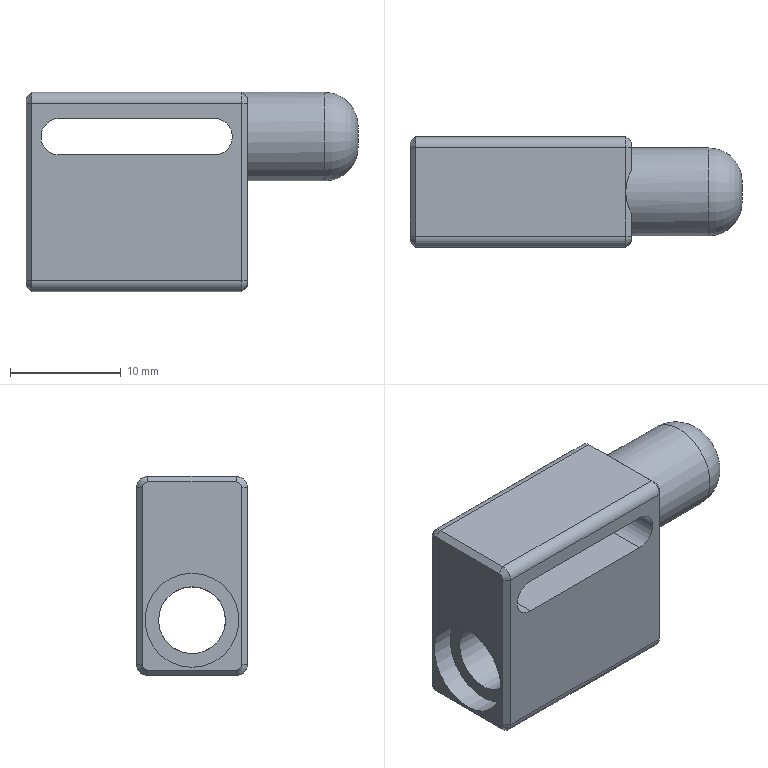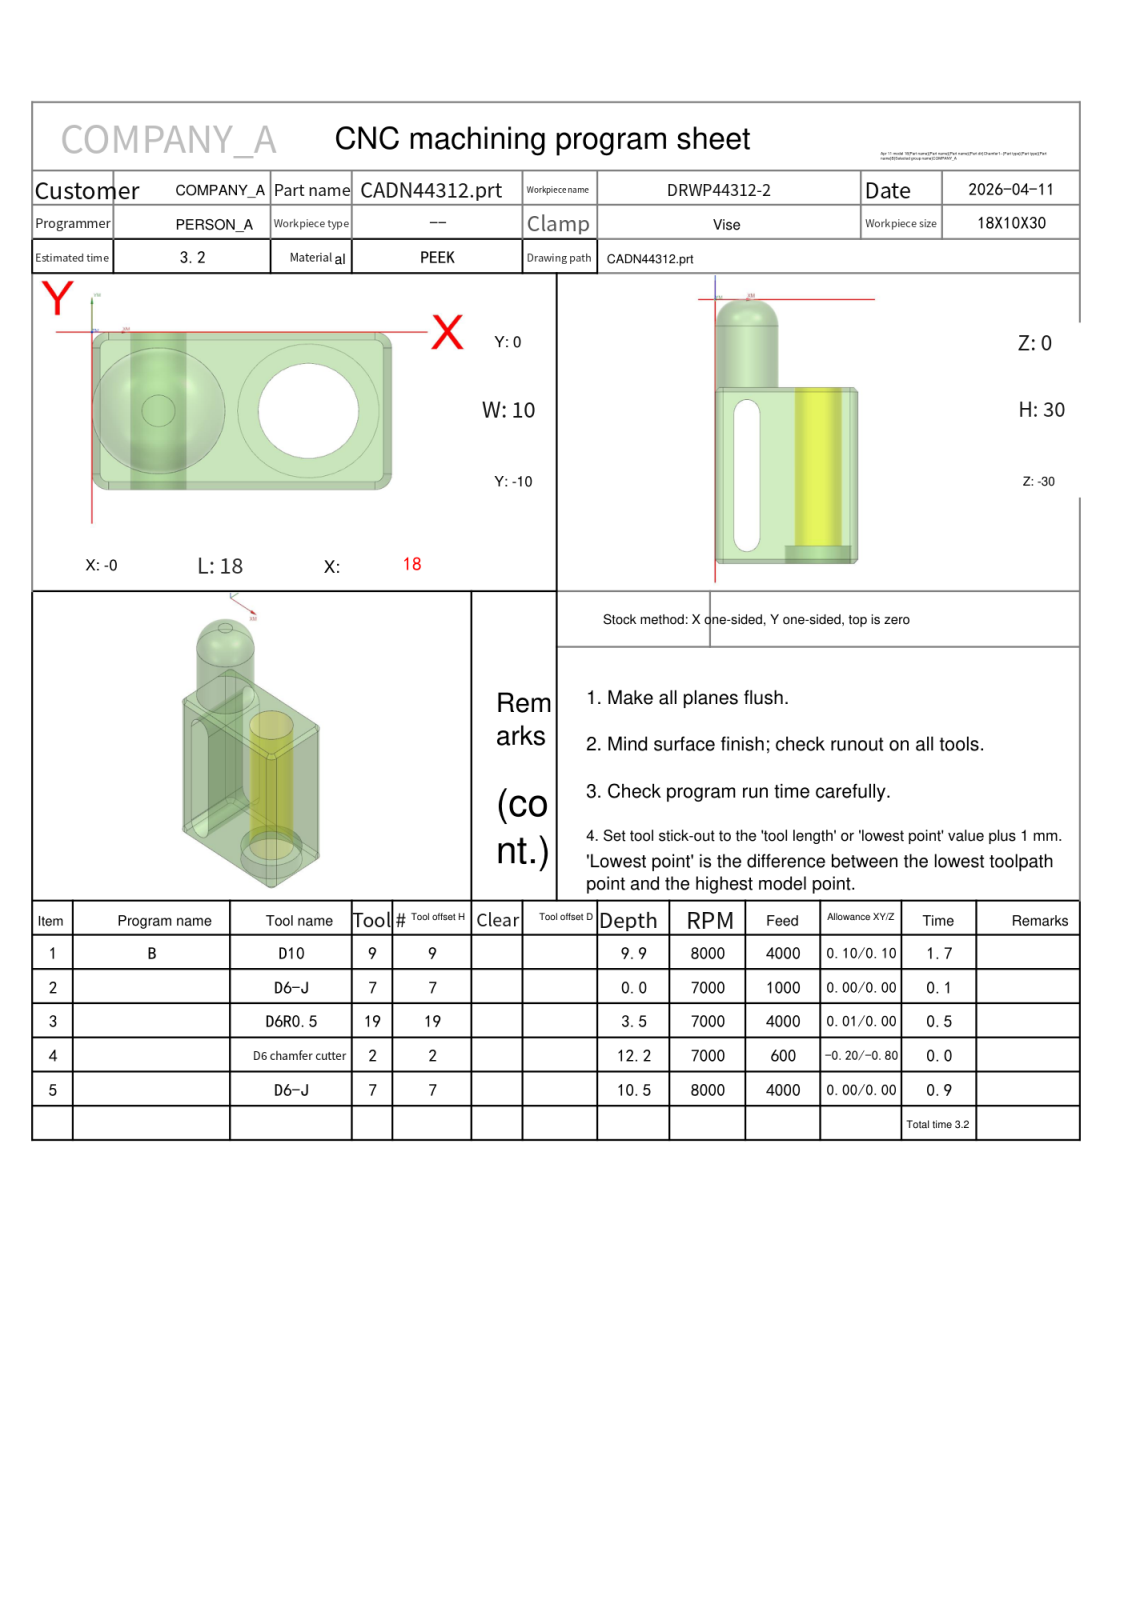NC program | NX | posted by the shop | part box 30 x 10 x 18 mm
Lines 1409 to 2960 of 11854:
N3 T19 M06
(D6R0.5  D=6. R=0.5 H=19 ce=0.01 di=0.00)
G00 G90 G54 X3.603 Y-8.689 M03 S7000
G43 H19 Z20.
M08
Z1.5
G01 X3.59 Y-8.688 Z1.499 F4000.
X3.069 Y-8.592 Z1.472
X2.568 Y-8.423 Z1.444
X2.096 Y-8.185 Z1.416
X1.662 Y-7.882 Z1.388
X1.276 Y-7.52 Z1.361
X.945 Y-7.107 Z1.333
X.743 Y-6.779 Z1.313
X.565 Y-6.404 Z1.291
X.43 Y-6.011 Z1.269
X.339 Y-5.606 Z1.247
X.294 Y-5.193 Z1.226
Y-4.807 Z1.205
X.353 Y-4.316 Z1.18
X.476 Y-3.836 Z1.154
X.663 Y-3.378 Z1.128
X.908 Y-2.948 Z1.102
X1.209 Y-2.555 Z1.076
X1.559 Y-2.205 Z1.05
X1.953 Y-1.905 Z1.024
X2.383 Y-1.66 Z.998
X2.842 Y-1.474 Z.972
X3.322 Y-1.352 Z.946
X3.704 Y-1.301 Z.926
X4.097 Y-1.29 Z.905
X4.489 Y-1.322 Z.885
X4.868 Y-1.392 Z.864
X5.352 Y-1.544 Z.838
X5.81 Y-1.76 Z.811
X6.234 Y-2.037 Z.785
X6.617 Y-2.369 Z.758
X6.951 Y-2.751 Z.732
X7.23 Y-3.174 Z.705
X7.449 Y-3.631 Z.678
X7.603 Y-4.114 Z.652
X7.691 Y-4.613 Z.625
X7.709 Y-5.119 Z.599
X7.658 Y-5.624 Z.572
X7.539 Y-6.116 Z.546
X7.354 Y-6.588 Z.519
X7.106 Y-7.03 Z.493
X6.879 Y-7.341 Z.472
X6.517 Y-7.727 Z.445
X6.103 Y-8.057 Z.417
X5.647 Y-8.325 Z.389
X5.158 Y-8.526 Z.361
X4.644 Y-8.654 Z.334
X4.118 Y-8.709 Z.306
X3.59 Y-8.688 Z.278
X3.069 Y-8.592 Z.251
X2.568 Y-8.423 Z.223
X2.096 Y-8.185 Z.195
X1.662 Y-7.882 Z.167
X1.276 Y-7.52 Z.14
X.945 Y-7.107 Z.112
X.743 Y-6.779 Z.092
X.565 Y-6.404 Z.07
X.43 Y-6.011 Z.048
X.339 Y-5.606 Z.026
X.294 Y-5.193 Z.005
Y-5. Z-.005
G02 X4. Y-1.294 I3.706 J0.0
X7.706 Y-5. I0.0 J-3.706
X4. Y-8.706 I-3.706 J0.0
X.294 Y-5. I0.0 J3.706
G01 X.295 Y-4.905 Z-.006
X.299 Y-4.81
X.304 Y-4.714
X.312 Y-4.62
X.322 Y-4.525
X.336 Y-4.431
X.35 Y-4.336
X.368 Y-4.243
X.388 Y-4.149
X.411 Y-4.057
X.435 Y-3.965
X.463 Y-3.873
X.492 Y-3.783
X.524 Y-3.693
X.558 Y-3.603
X.595 Y-3.516
X.633 Y-3.428
X.675 Y-3.342
X.718 Y-3.257
X.763 Y-3.173
X.81 Y-3.09
X.86 Y-3.008
X.912 Y-2.928
X.966 Y-2.849
X1.022 Y-2.771
X1.08 Y-2.695
X1.139 Y-2.62
X1.201 Y-2.548
X1.264 Y-2.476
X1.33 Y-2.406
X1.397 Y-2.338 Z-.007
X1.466 Y-2.272
X1.536 Y-2.207
X1.608 Y-2.144
X1.682 Y-2.083
X1.758 Y-2.024
X1.835 Y-1.967
X1.913 Y-1.912
X1.993 Y-1.859
X2.074 Y-1.808
X2.156 Y-1.759
X2.24 Y-1.713
X2.325 Y-1.668
X2.411 Y-1.626
X2.498 Y-1.585
X2.586 Y-1.547
X2.675 Y-1.511
X2.765 Y-1.478
X2.855 Y-1.447
X2.947 Y-1.419
X3.039 Y-1.392
X3.132 Y-1.368
X3.225 Y-1.346
X3.32 Y-1.328
X3.421 Y-1.309
X3.524 Y-1.294
X3.663 Y-1.278
X3.803 Y-1.268
X3.95 Y-1.262 Z-.008
X4.098
X4.246 Y-1.268
X4.393 Y-1.28
X4.54 Y-1.297
X4.685 Y-1.321
X4.778 Y-1.339
X4.87 Y-1.359
X4.962 Y-1.382
X5.053 Y-1.407
X5.089 Y-1.417
X5.125 Y-1.428
X5.269 Y-1.476
X5.41 Y-1.529
X5.498 Y-1.565
X5.584 Y-1.604
X5.669 Y-1.644
X5.753 Y-1.687
X5.919 Y-1.779
X6.079 Y-1.879
X6.235 Y-1.987
X6.384 Y-2.103
X6.528 Y-2.226
X6.665 Y-2.356 Z-.009
X6.796 Y-2.493
X6.919 Y-2.637
X7.036 Y-2.787
X7.144 Y-2.942
X7.245 Y-3.103
X7.337 Y-3.268
X7.421 Y-3.438
X7.496 Y-3.612
X7.562 Y-3.79
X7.62 Y-3.971
X7.668 Y-4.155
X7.707 Y-4.34
X7.736 Y-4.528
X7.756 Y-4.717
X7.767 Y-4.907 Z-.01
Y-5.097
X7.759 Y-5.287
X7.74 Y-5.476
X7.712 Y-5.664
X7.675 Y-5.85
X7.628 Y-6.035
X7.572 Y-6.217
X7.507 Y-6.396
X7.433 Y-6.571
X7.393 Y-6.657
X7.351 Y-6.743
X7.306 Y-6.827
X7.259 Y-6.909
X7.193 Y-7.02
X7.123 Y-7.127
X7.088 Y-7.179
X7.052 Y-7.229
X6.994 Y-7.308
X6.933 Y-7.384
X6.872 Y-7.459
X6.807 Y-7.532 Z-.011
X6.742 Y-7.605
X6.674 Y-7.674
X6.604 Y-7.743
X6.533 Y-7.809
X6.46 Y-7.874
X6.385 Y-7.937
X6.309 Y-7.998
X6.231 Y-8.056
X6.152 Y-8.114
X6.071 Y-8.168
X5.99 Y-8.221
X5.906 Y-8.271
X5.821 Y-8.32
X5.735 Y-8.366
X5.648 Y-8.41
X5.56 Y-8.452
X5.471 Y-8.491
X5.38 Y-8.528
X5.289 Y-8.563
X5.197 Y-8.595
X5.104 Y-8.626
X5.01 Y-8.653
X4.916 Y-8.679
X4.821 Y-8.701
X4.725 Y-8.722
X4.629 Y-8.739
X4.533 Y-8.755
X4.436 Y-8.768
X4.339 Y-8.778 Z-.012
X4.241 Y-8.786
X4.144 Y-8.792
X4.046 Y-8.794
X3.948 Y-8.795
X3.85 Y-8.793
X3.752 Y-8.788
X3.655 Y-8.781
X3.557 Y-8.771
X3.46 Y-8.759
X3.364 Y-8.744
X3.267 Y-8.727
X3.171 Y-8.707
X3.076 Y-8.685
X2.981 Y-8.66
X2.887 Y-8.633
X2.794 Y-8.604
X2.701 Y-8.572
X2.609 Y-8.538
X2.519 Y-8.501
X2.429 Y-8.462
X2.34 Y-8.421
X2.252 Y-8.377
X2.165 Y-8.331
X2.08 Y-8.283
X1.996 Y-8.233
X1.913 Y-8.181
X1.831 Y-8.126
X1.751 Y-8.07
X1.673 Y-8.011 Z-.013
X1.596 Y-7.95
X1.52 Y-7.887
X1.446 Y-7.823
X1.374 Y-7.756
X1.304 Y-7.688
X1.235 Y-7.618
X1.168 Y-7.546
X1.103 Y-7.472
X1.04 Y-7.397
X.979 Y-7.32
X.92 Y-7.242
X.863 Y-7.162
X.808 Y-7.081
X.755 Y-6.998
X.737 Y-6.969
X.719 Y-6.939
X.649 Y-6.817
X.584 Y-6.692
X.509 Y-6.534
X.442 Y-6.372
X.382 Y-6.207
X.33 Y-6.039
X.285 Y-5.87
X.248 Y-5.698
X.219 Y-5.525 Z-.014
X.199 Y-5.351
X.185 Y-5.176
X.18 Y-5.
X.184 Y-4.816
X.197 Y-4.633
X.218 Y-4.45
X.248 Y-4.269
X.286 Y-4.089
X.334 Y-3.912
X.389 Y-3.736
X.453 Y-3.564
X.526 Y-3.394
X.606 Y-3.229 Z-.015
X.694 Y-3.067
X.79 Y-2.91
X.894 Y-2.758
X1.004 Y-2.61
X1.122 Y-2.468
X1.246 Y-2.332
X1.377 Y-2.202
X1.514 Y-2.079
X1.657 Y-1.962
X1.805 Y-1.852
X1.959 Y-1.749
X2.117 Y-1.654 Z-.016
X2.28 Y-1.567
X2.446 Y-1.487
X2.617 Y-1.416
X2.79 Y-1.353
X2.967 Y-1.298
X3.146 Y-1.252
X3.302 Y-1.219
X3.46 Y-1.192
X3.485 Y-1.188
X3.51 Y-1.185
X3.675 Y-1.167
X3.841 Y-1.156
X4.008 Y-1.151
X4.174 Y-1.155 Z-.017
X4.341 Y-1.165
X4.506 Y-1.183
X4.524 Y-1.186
X4.541 Y-1.187
X4.689 Y-1.21
X4.835 Y-1.24
X4.997 Y-1.278
X5.158 Y-1.324
X5.337 Y-1.385
X5.513 Y-1.454
X5.685 Y-1.531
X5.854 Y-1.617
X6.018 Y-1.712
X6.177 Y-1.814
X6.331 Y-1.924 Z-.018
X6.48 Y-2.041
X6.622 Y-2.165
X6.759 Y-2.297
X6.889 Y-2.435
X7.011 Y-2.579
X7.127 Y-2.729
X7.236 Y-2.885
X7.336 Y-3.045
X7.429 Y-3.211
X7.513 Y-3.381
X7.589 Y-3.555
X7.656 Y-3.732 Z-.019
X7.715 Y-3.912
X7.764 Y-4.096
X7.805 Y-4.281
X7.837 Y-4.469
X7.859 Y-4.657
X7.872 Y-4.847
X7.876 Y-5.037
X7.87 Y-5.227
X7.855 Y-5.416
X7.831 Y-5.605
X7.797 Y-5.792 Z-.02
X7.754 Y-5.978
X7.703 Y-6.161
X7.642 Y-6.341
X7.573 Y-6.518
X7.495 Y-6.692
X7.408 Y-6.862
X7.387 Y-6.902
X7.364 Y-6.941
X7.29 Y-7.066
X7.211 Y-7.187
X7.155 Y-7.268
X7.098 Y-7.347
X7.038 Y-7.424
X6.976 Y-7.5
X6.913 Y-7.574
X6.848 Y-7.647
X6.781 Y-7.718 Z-.021
X6.712 Y-7.787
X6.641 Y-7.855
X6.569 Y-7.92
X6.495 Y-7.984
X6.419 Y-8.046
X6.343 Y-8.106
X6.264 Y-8.165
X6.184 Y-8.221
X6.103 Y-8.275
X6.02 Y-8.327
X5.936 Y-8.377
X5.851 Y-8.425
X5.764 Y-8.471
X5.677 Y-8.514
X5.588 Y-8.556
X5.498 Y-8.595
X5.408 Y-8.632
X5.316 Y-8.666
X5.224 Y-8.699
X5.131 Y-8.729
X5.037 Y-8.756
X4.942 Y-8.782
X4.847 Y-8.804 Z-.022
X4.751 Y-8.825
X4.655 Y-8.843
X4.558 Y-8.859
X4.461 Y-8.872
X4.364 Y-8.882
X4.266 Y-8.891
X4.168 Y-8.897
X4.07 Y-8.9
X3.972 Y-8.901
X3.874 Y-8.899
X3.776 Y-8.895
X3.679 Y-8.889
X3.581 Y-8.88
X3.484 Y-8.869
X3.387 Y-8.855
X3.29 Y-8.839
X3.194 Y-8.82
X3.098 Y-8.799
X2.908 Y-8.75
X2.721 Y-8.691 Z-.023
X2.537 Y-8.622
X2.356 Y-8.545
X2.18 Y-8.459
X2.008 Y-8.364
X1.841 Y-8.26
X1.68 Y-8.148
X1.524 Y-8.028
X1.375 Y-7.901
X1.232 Y-7.766
X1.096 Y-7.624
X1.03 Y-7.55
X.967 Y-7.475
X.906 Y-7.398 Z-.024
X.846 Y-7.32
X.796 Y-7.251
X.748 Y-7.181
X.686 Y-7.088
X.628 Y-6.992
X.542 Y-6.841
X.463 Y-6.686
X.391 Y-6.527
X.326 Y-6.365
X.268 Y-6.201
X.218 Y-6.034
X.175 Y-5.865
X.14 Y-5.694
X.112 Y-5.522
X.092 Y-5.348 Z-.025
X.08 Y-5.174
X.075 Y-5.
X.079 Y-4.813
X.092 Y-4.626
X.113 Y-4.44
X.143 Y-4.256
X.182 Y-4.072
X.23 Y-3.891
X.286 Y-3.713
X.351 Y-3.537 Z-.026
X.424 Y-3.364
X.505 Y-3.195
X.594 Y-3.031
X.691 Y-2.87
X.796 Y-2.714
X.908 Y-2.564
X1.027 Y-2.419
X1.152 Y-2.279
X1.285 Y-2.146
X1.423 Y-2.019 Z-.027
X1.568 Y-1.899
X1.717 Y-1.786
X1.873 Y-1.68
X2.033 Y-1.582
X2.198 Y-1.492
X2.366 Y-1.409
X2.539 Y-1.334
X2.715 Y-1.268
X2.894 Y-1.21
X3.076 Y-1.161 Z-.028
X3.26 Y-1.121
X3.445 Y-1.089
X3.484 Y-1.083
X3.522 Y-1.079
X3.668 Y-1.063
X3.814 Y-1.053
X4. Y-1.047
X4.186 Y-1.051
X4.371 Y-1.063
X4.556 Y-1.084
X4.746 Y-1.115 Z-.029
X4.935 Y-1.156
X4.989 Y-1.168
X5.042 Y-1.183
X5.175 Y-1.221
X5.306 Y-1.264
X5.487 Y-1.331
X5.665 Y-1.407
X5.839 Y-1.492
X6.008 Y-1.585
X6.173 Y-1.686
X6.332 Y-1.796 Z-.03
X6.487 Y-1.913
X6.635 Y-2.037
X6.777 Y-2.169
X6.912 Y-2.307
X7.041 Y-2.452
X7.162 Y-2.603
X7.276 Y-2.76
X7.382 Y-2.922
X7.481 Y-3.089
X7.57 Y-3.261 Z-.031
X7.652 Y-3.437
X7.725 Y-3.617
X7.788 Y-3.8
X7.843 Y-3.986
X7.889 Y-4.175
X7.926 Y-4.365
X7.953 Y-4.558
X7.97 Y-4.751
X7.978 Y-4.945 Z-.032
X7.977 Y-5.14
X7.966 Y-5.334
X7.946 Y-5.527
X7.916 Y-5.719
X7.877 Y-5.909
X7.829 Y-6.098
X7.772 Y-6.284
X7.705 Y-6.467
X7.63 Y-6.646 Z-.033
X7.546 Y-6.822
X7.454 Y-6.993
X7.411 Y-7.067
X7.366 Y-7.139
X7.308 Y-7.229
X7.247 Y-7.317
X7.132 Y-7.472
X7.009 Y-7.621
X6.88 Y-7.763
X6.744 Y-7.9
X6.601 Y-8.029
X6.452 Y-8.152 Z-.034
X6.298 Y-8.267
X6.138 Y-8.375
X5.973 Y-8.475
X5.803 Y-8.566
X5.629 Y-8.65
X5.452 Y-8.725
X5.27 Y-8.792
X5.086 Y-8.849
X4.899 Y-8.898 Z-.035
X4.71 Y-8.937
X4.52 Y-8.968
X4.328 Y-8.989
X4.135 Y-9.001
X3.941 Y-9.004
X3.748 Y-8.997
X3.556 Y-8.981
X3.364 Y-8.956
X3.174 Y-8.921 Z-.036
X2.985 Y-8.877
X2.799 Y-8.825
X2.616 Y-8.763
X2.435 Y-8.692
X2.259 Y-8.613
X2.086 Y-8.526
X1.918 Y-8.43
X1.754 Y-8.326
X1.596 Y-8.214
X1.443 Y-8.095 Z-.037
X1.296 Y-7.969
X1.156 Y-7.835
X1.021 Y-7.695
X.894 Y-7.549
X.774 Y-7.396
X.662 Y-7.238
X.643 Y-7.21
X.624 Y-7.181
X.537 Y-7.042
X.457 Y-6.9
X.367 Y-6.724 Z-.038
X.286 Y-6.543
X.248 Y-6.451
X.214 Y-6.359
X.181 Y-6.265
X.151 Y-6.171
X.123 Y-6.076
X.097 Y-5.98
X.074 Y-5.884
X.053 Y-5.787
X.034 Y-5.69
X.018 Y-5.592
X.004 Y-5.494
X-.007 Y-5.396
X-.022 Y-5.198
X-.028 Y-5. Z-.039
X-.024 Y-4.805
X-.011 Y-4.611
X.012 Y-4.418
X.044 Y-4.226
X.085 Y-4.035
X.135 Y-3.847
X.195 Y-3.661
X.263 Y-3.479 Z-.04
X.34 Y-3.3
X.426 Y-3.125
X.52 Y-2.954
X.622 Y-2.788
X.732 Y-2.626
X.85 Y-2.471
X.975 Y-2.321
X1.107 Y-2.178 Z-.041
X1.247 Y-2.041
X1.392 Y-1.91
X1.544 Y-1.787
X1.702 Y-1.672
X1.865 Y-1.564
X2.033 Y-1.464
X2.205 Y-1.373
X2.382 Y-1.289 Z-.042
X2.563 Y-1.215
X2.747 Y-1.149
X2.935 Y-1.092
X3.124 Y-1.045
X3.316 Y-1.006
X3.51 Y-.977
X3.705 Y-.957
X3.901 Y-.947 Z-.043
X4.098 Y-.946
X4.294 Y-.955
X4.49 Y-.973
X4.684 Y-1.001
X4.878 Y-1.038
X5.069 Y-1.084
X5.222 Y-1.128
X5.373 Y-1.179 Z-.044
X5.411 Y-1.192
X5.449 Y-1.207
X5.542 Y-1.243
X5.634 Y-1.282
X5.725 Y-1.322
X5.816 Y-1.366
X5.905 Y-1.411
X5.993 Y-1.459
X6.079 Y-1.508
X6.165 Y-1.561
X6.249 Y-1.614
X6.332 Y-1.671
X6.414 Y-1.728
X6.493 Y-1.789
X6.572 Y-1.851
X6.649 Y-1.915 Z-.045
X6.724 Y-1.98
X6.798 Y-2.048
X6.87 Y-2.117
X6.941 Y-2.189
X7.009 Y-2.262
X7.076 Y-2.336
X7.141 Y-2.413
X7.204 Y-2.491
X7.265 Y-2.57
X7.324 Y-2.651
X7.381 Y-2.733
X7.436 Y-2.817
X7.49 Y-2.902
X7.54 Y-2.988
X7.589 Y-3.076 Z-.046
X7.636 Y-3.164
X7.68 Y-3.254
X7.723 Y-3.345
X7.763 Y-3.437
X7.8 Y-3.53
X7.836 Y-3.624
X7.869 Y-3.719
X7.9 Y-3.814
X7.928 Y-3.91
X7.954 Y-4.007
X7.978 Y-4.105
X7.999 Y-4.203
X8.018 Y-4.301
X8.034 Y-4.4
X8.048 Y-4.5 Z-.047
X8.059 Y-4.599
X8.068 Y-4.699
X8.075 Y-4.8
X8.079 Y-4.9
X8.081 Y-5.
X8.08 Y-5.101
X8.076 Y-5.201
X8.071 Y-5.302
X8.062 Y-5.402
X8.052 Y-5.502
X8.039 Y-5.601
X8.023 Y-5.7
X8.005 Y-5.799
X7.984 Y-5.898
X7.961 Y-5.996
X7.936 Y-6.093 Z-.048
X7.908 Y-6.19
X7.878 Y-6.285
X7.846 Y-6.381
X7.811 Y-6.475
X7.774 Y-6.569
X7.734 Y-6.661
X7.693 Y-6.753
X7.649 Y-6.843
X7.563 Y-7.006
X7.469 Y-7.165
X7.46 Y-7.179
X7.451 Y-7.194
X7.344 Y-7.356
X7.228 Y-7.513 Z-.049
X7.105 Y-7.665
X6.975 Y-7.81
X6.839 Y-7.949
X6.695 Y-8.082
X6.546 Y-8.207
X6.391 Y-8.325
X6.23 Y-8.436
X6.064 Y-8.539 Z-.05
X5.893 Y-8.634
X5.718 Y-8.721
X5.539 Y-8.799
X5.357 Y-8.869
X5.171 Y-8.93
X4.983 Y-8.982
X4.792 Y-9.025
X4.6 Y-9.059 Z-.051
X4.406 Y-9.084
X4.211 Y-9.099
X4.015 Y-9.105
X3.82 Y-9.102
X3.624 Y-9.09
X3.43 Y-9.068
X3.236 Y-9.037 Z-.052
X3.045 Y-8.996
X2.855 Y-8.947
X2.668 Y-8.889
X2.484 Y-8.822
X2.304 Y-8.746
X2.127 Y-8.661
X1.954 Y-8.568
X1.786 Y-8.468 Z-.053
X1.623 Y-8.359
X1.465 Y-8.242
X1.313 Y-8.118
X1.167 Y-7.987
X1.027 Y-7.849
X.894 Y-7.705
X.769 Y-7.554
X.65 Y-7.398 Z-.054
X.539 Y-7.236
X.521 Y-7.209
X.504 Y-7.181
X.419 Y-7.04
X.34 Y-6.896
X.253 Y-6.719
X.174 Y-6.539
X.105 Y-6.354
X.044 Y-6.167
X-.008 Y-5.977 Z-.055
X-.051 Y-5.784
X-.085 Y-5.59
X-.109 Y-5.394
X-.124 Y-5.197
X-.129 Y-5.
X-.125 Y-4.8
X-.111 Y-4.601 Z-.056
X-.088 Y-4.402
X-.055 Y-4.205
X-.013 Y-4.009
X.039 Y-3.816
X.1 Y-3.625
X.171 Y-3.438
X.25 Y-3.254 Z-.057
X.338 Y-3.074
X.435 Y-2.899
X.54 Y-2.728
X.654 Y-2.563
X.775 Y-2.403
X.904 Y-2.25
X1.04 Y-2.102 Z-.058
X1.183 Y-1.962
X1.333 Y-1.829
X1.489 Y-1.703
X1.651 Y-1.584
X1.819 Y-1.474
X1.992 Y-1.372
X2.169 Y-1.278 Z-.059
X2.351 Y-1.193
X2.537 Y-1.117
X2.726 Y-1.05
X2.919 Y-.992
X3.114 Y-.944
X3.212 Y-.923
X3.311 Y-.905 Z-.06
X3.41 Y-.889
X3.51 Y-.876
X3.702 Y-.857
X3.894 Y-.846
X4.086 Y-.845
X4.278 Y-.853
X4.47 Y-.869
X4.661 Y-.895 Z-.061
X4.781 Y-.915
X4.901 Y-.94
X4.97 Y-.955
X5.038 Y-.972
X5.224 Y-1.024
X5.407 Y-1.084
X5.59 Y-1.154
X5.769 Y-1.232
X5.944 Y-1.318 Z-.062
X6.115 Y-1.413
X6.281 Y-1.515
X6.443 Y-1.626
X6.599 Y-1.743
X6.749 Y-1.868
X6.894 Y-2.
X7.032 Y-2.139 Z-.063
X7.163 Y-2.284
X7.288 Y-2.435
X7.405 Y-2.591
X7.515 Y-2.753
X7.617 Y-2.92
X7.712 Y-3.092
X7.798 Y-3.268 Z-.064
X7.875 Y-3.448
X7.945 Y-3.631
X8.005 Y-3.818
X8.057 Y-4.007
X8.1 Y-4.198
X8.134 Y-4.391
X8.159 Y-4.586 Z-.065
X8.174 Y-4.781
X8.181 Y-4.977
X8.178 Y-5.174
X8.166 Y-5.369
X8.145 Y-5.565
X8.114 Y-5.759
X8.075 Y-5.951 Z-.066
X8.027 Y-6.141
X7.969 Y-6.329
X7.903 Y-6.514
X7.829 Y-6.696
X7.745 Y-6.874
X7.654 Y-7.048
X7.554 Y-7.218 Z-.067
X7.494 Y-7.313
X7.43 Y-7.406
X7.379 Y-7.479
X7.325 Y-7.551
X7.263 Y-7.631
X7.199 Y-7.709
X7.133 Y-7.785
X7.065 Y-7.86
X6.996 Y-7.934
X6.924 Y-8.005
X6.851 Y-8.075
X6.777 Y-8.143 Z-.068
X6.7 Y-8.21
X6.622 Y-8.274
X6.543 Y-8.337
X6.462 Y-8.397
X6.379 Y-8.456
X6.296 Y-8.513
X6.21 Y-8.568
X6.124 Y-8.62
X6.036 Y-8.671
X5.947 Y-8.719
X5.857 Y-8.765
X5.766 Y-8.809
X5.674 Y-8.851 Z-.069
X5.581 Y-8.891
X5.486 Y-8.928
X5.391 Y-8.963
X5.295 Y-8.996
X5.199 Y-9.026
X5.102 Y-9.054
X5.004 Y-9.08
X4.905 Y-9.103
X4.806 Y-9.124
X4.706 Y-9.143
X4.606 Y-9.159
X4.506 Y-9.173
X4.405 Y-9.184
X4.304 Y-9.193 Z-.07
X4.203 Y-9.2
X4.101 Y-9.204
X4. Y-9.205
X3.899
X3.797 Y-9.201
X3.696 Y-9.196
X3.595 Y-9.187
X3.494 Y-9.177
X3.393 Y-9.164
X3.193 Y-9.13
X2.995 Y-9.087 Z-.071
X2.799 Y-9.035
X2.605 Y-8.973
X2.415 Y-8.902
X2.228 Y-8.821
X2.046 Y-8.732
X1.868 Y-8.634
X1.695 Y-8.528 Z-.072
X1.527 Y-8.413
X1.365 Y-8.29
X1.209 Y-8.16
X1.059 Y-8.022
X.916 Y-7.878
X.78 Y-7.726 Z-.073
X.652 Y-7.568
X.532 Y-7.404
X.419 Y-7.234
X.403 Y-7.208
X.386 Y-7.182
X.303 Y-7.039
X.226 Y-6.893
X.141 Y-6.716
X.065 Y-6.535 Z-.074
X-.003 Y-6.35
X-.062 Y-6.163
X-.112 Y-5.973
X-.153 Y-5.781
X-.186 Y-5.588
X-.209 Y-5.393
X-.224 Y-5.196 Z-.075
X-.229 Y-5.
X-.228 Y-4.897
X-.225 Y-4.795
X-.219 Y-4.692
X-.211 Y-4.59
X-.2 Y-4.488
X-.187 Y-4.386
X-.171 Y-4.285
X-.153 Y-4.184
X-.132 Y-4.083
X-.109 Y-3.983 Z-.076
X-.084 Y-3.884
X-.056 Y-3.785
X-.026 Y-3.687
X.007 Y-3.589
X.042 Y-3.493
X.079 Y-3.397
X.119 Y-3.302
X.161 Y-3.209
X.205 Y-3.116
X.252 Y-3.024
X.3 Y-2.934
X.351 Y-2.844 Z-.077
X.404 Y-2.756
X.459 Y-2.669
X.517 Y-2.584
X.576 Y-2.5
X.637 Y-2.417
X.7 Y-2.336
X.766 Y-2.257
X.833 Y-2.179
X.902 Y-2.103
X.973 Y-2.028
X1.046 Y-1.955 Z-.078
X1.12 Y-1.884
X1.196 Y-1.815
X1.274 Y-1.748
X1.353 Y-1.682
X1.434 Y-1.619
X1.517 Y-1.557
X1.601 Y-1.498
X1.686 Y-1.44
X1.773 Y-1.385
X1.861 Y-1.331
X1.951 Y-1.28
X2.041 Y-1.231 Z-.079
X2.133 Y-1.185
X2.226 Y-1.14
X2.32 Y-1.098
X2.415 Y-1.058
X2.511 Y-1.02
X2.608 Y-.985
X2.706 Y-.952
X2.804 Y-.921
X2.903 Y-.893
X3.003 Y-.867
X3.104 Y-.844
X3.205 Y-.823 Z-.08
X3.306 Y-.805
X3.414 Y-.788
X3.521 Y-.774
X3.692 Y-.757
X3.864 Y-.748
X4.041 Y-.745
X4.219 Y-.75
X4.396 Y-.762 Z-.081
X4.572 Y-.782
X4.748 Y-.808
X4.922 Y-.843
X5.101 Y-.886
X5.278 Y-.936
X5.293 Y-.941
X5.307 Y-.946
X5.495 Y-1.01 Z-.082
X5.681 Y-1.084
X5.862 Y-1.166
X6.04 Y-1.257
X6.213 Y-1.355
X6.381 Y-1.462
X6.545 Y-1.577
X6.702 Y-1.699 Z-.083
X6.854 Y-1.828
X7. Y-1.965
X7.139 Y-2.108
X7.271 Y-2.257
X7.397 Y-2.413
X7.514 Y-2.574 Z-.084
X7.625 Y-2.74
X7.727 Y-2.912
X7.821 Y-3.088
X7.907 Y-3.269
X7.984 Y-3.453
X8.053 Y-3.641 Z-.085
X8.113 Y-3.831
X8.164 Y-4.025
X8.206 Y-4.22
X8.238 Y-4.418
X8.261 Y-4.616
X8.276 Y-4.816 Z-.086
X8.28 Y-5.016
X8.275 Y-5.216
X8.261 Y-5.416
X8.238 Y-5.615
X8.205 Y-5.812
X8.163 Y-6.008 Z-.087
X8.113 Y-6.202
X8.052 Y-6.393
X7.984 Y-6.581
X7.906 Y-6.766
X7.82 Y-6.947
X7.725 Y-7.124 Z-.088
X7.641 Y-7.267
X7.55 Y-7.407
X7.531 Y-7.435
X7.512 Y-7.463
X7.392 Y-7.627
X7.264 Y-7.785
X7.13 Y-7.937
X6.988 Y-8.082 Z-.089
X6.839 Y-8.221
X6.684 Y-8.352
X6.523 Y-8.476
X6.356 Y-8.591
X6.184 Y-8.7
X6.007 Y-8.799 Z-.09
X5.826 Y-8.891
X5.64 Y-8.973
X5.45 Y-9.047
X5.258 Y-9.112
X5.062 Y-9.167
X4.864 Y-9.214 Z-.091
X4.664 Y-9.251
X4.462 Y-9.278
X4.259 Y-9.296
X4.056 Y-9.304
X3.852 Y-9.302 Z-.092
X3.649 Y-9.291
X3.446 Y-9.271
X3.245 Y-9.24
X3.045 Y-9.201
X2.847 Y-9.152
X2.652 Y-9.093 Z-.093
X2.46 Y-9.025
X2.271 Y-8.949
X2.086 Y-8.863
X1.905 Y-8.769
X1.729 Y-8.666
X1.558 Y-8.556 Z-.094
X1.392 Y-8.437
X1.232 Y-8.31
X1.078 Y-8.176
X.93 Y-8.035
X.79 Y-7.887
X.656 Y-7.732 Z-.095
X.53 Y-7.571
X.412 Y-7.405
X.302 Y-7.233
X.286 Y-7.207
X.271 Y-7.182
X.19 Y-7.037
X.114 Y-6.89
X.032 Y-6.712 Z-.096
X-.042 Y-6.531
X-.108 Y-6.347
X-.166 Y-6.16
X-.215 Y-5.97
X-.255 Y-5.779
X-.286 Y-5.586 Z-.097
X-.309 Y-5.391
X-.323 Y-5.196
X-.328 Y-5.
X-.324 Y-4.803
X-.312 Y-4.606
X-.29 Y-4.41 Z-.098
X-.259 Y-4.215
X-.22 Y-4.022
X-.172 Y-3.83
X-.115 Y-3.641
X-.049 Y-3.455
X.024 Y-3.272 Z-.099
X.107 Y-3.092
X.197 Y-2.916
X.295 Y-2.745
X.401 Y-2.578
X.515 Y-2.416 Z-.1
X.635 Y-2.26
X.763 Y-2.109
X.898 Y-1.964
X1.038 Y-1.825
X1.186 Y-1.693
X1.339 Y-1.568 Z-.101
X1.498 Y-1.449
X1.661 Y-1.339
X1.83 Y-1.235
X2.004 Y-1.14
X2.181 Y-1.052 Z-.102
X2.363 Y-.973
X2.548 Y-.902
X2.736 Y-.839
X2.926 Y-.785
X3.119 Y-.74
X3.219 Y-.72
X3.319 Y-.703 Z-.103
X3.415 Y-.688
X3.51 Y-.676
X3.691 Y-.659
X3.873 Y-.649
X4.054 Y-.647
X4.236 Y-.652
X4.417 Y-.665 Z-.104
X4.598 Y-.686
X4.64 Y-.691
X4.681 Y-.698
X4.819 Y-.721
X4.956 Y-.749
X5.133 Y-.792
X5.308 Y-.842
X5.5 Y-.907 Z-.105
X5.689 Y-.981
X5.875 Y-1.063
X6.056 Y-1.154
X6.233 Y-1.253
X6.405 Y-1.36 Z-.106
X6.573 Y-1.475
X6.734 Y-1.598
X6.89 Y-1.729
X7.04 Y-1.866
X7.183 Y-2.011
X7.319 Y-2.162 Z-.107
X7.448 Y-2.319
X7.57 Y-2.481
X7.684 Y-2.65
X7.79 Y-2.823
X7.888 Y-3.002 Z-.108
X7.977 Y-3.185
X8.058 Y-3.371
X8.13 Y-3.562
X8.193 Y-3.755
X8.247 Y-3.951
X8.292 Y-4.15 Z-.109
X8.328 Y-4.35
X8.354 Y-4.553
X8.371 Y-4.755
X8.378 Y-4.959
X8.376 Y-5.163 Z-.11
X8.364 Y-5.366
X8.343 Y-5.569
X8.313 Y-5.771
X8.273 Y-5.971
X8.224 Y-6.169 Z-.111
X8.166 Y-6.364
X8.098 Y-6.557
X8.022 Y-6.746
X7.937 Y-6.932
X7.844 Y-7.113
X7.759 Y-7.262 Z-.112
X7.668 Y-7.407
X7.65 Y-7.435
X7.632 Y-7.462
X7.572 Y-7.549
X7.51 Y-7.634
X7.446 Y-7.718
X7.38 Y-7.8
X7.312 Y-7.88
X7.242 Y-7.959
X7.171 Y-8.037 Z-.113
X7.097 Y-8.112
X7.022 Y-8.186
X6.945 Y-8.258
X6.866 Y-8.328
X6.785 Y-8.396
X6.703 Y-8.462
X6.62 Y-8.526
X6.535 Y-8.588
X6.448 Y-8.648
X6.36 Y-8.706
X6.27 Y-8.762 Z-.114
X6.18 Y-8.816
X6.087 Y-8.867
X5.994 Y-8.917
X5.9 Y-8.964
X5.804 Y-9.009
X5.708 Y-9.051
X5.61 Y-9.091
X5.511 Y-9.129
X5.412 Y-9.165
X5.312 Y-9.198 Z-.115
X5.211 Y-9.228
X5.109 Y-9.256
X5.007 Y-9.282
X4.904 Y-9.305
X4.8 Y-9.326
X4.696 Y-9.345
X4.592 Y-9.361
X4.487 Y-9.374
X4.382 Y-9.385
X4.276 Y-9.393
X4.171 Y-9.399 Z-.116
X4.065 Y-9.402
X3.96 Y-9.403
X3.854 Y-9.401
X3.748 Y-9.396
X3.643 Y-9.389
X3.538 Y-9.38
X3.433 Y-9.368
X3.328 Y-9.353
X3.223 Y-9.336
X3.119 Y-9.317 Z-.117
X3.016 Y-9.295
X2.913 Y-9.27
X2.811 Y-9.243
X2.709 Y-9.214
X2.608 Y-9.182
X2.508 Y-9.148
X2.409 Y-9.111
X2.311 Y-9.072
X2.213 Y-9.031
X2.117 Y-8.987 Z-.118
X2.022 Y-8.941
X1.927 Y-8.893
X1.834 Y-8.842
X1.743 Y-8.789
X1.652 Y-8.734
X1.563 Y-8.677
X1.475 Y-8.618
X1.389 Y-8.557
X1.304 Y-8.493
X1.221 Y-8.428
X1.139 Y-8.36 Z-.119
X1.059 Y-8.291
X.98 Y-8.22
X.904 Y-8.146
X.829 Y-8.072
X.756 Y-7.995
X.685 Y-7.916
X.615 Y-7.836
X.548 Y-7.754
X.483 Y-7.671
X.419 Y-7.586 Z-.12
X.362 Y-7.506
X.307 Y-7.424
X.245 Y-7.328
X.187 Y-7.231
X.091 Y-7.061
X.004 Y-6.887
X-.076 Y-6.709
X-.148 Y-6.528 Z-.121
X-.212 Y-6.344
X-.268 Y-6.157
X-.316 Y-5.968
X-.355 Y-5.777
X-.386 Y-5.584 Z-.122
X-.408 Y-5.39
X-.421 Y-5.195
X-.426 Y-5.
X-.425 Y-4.896
X-.422 Y-4.791
X-.416 Y-4.687
X-.408 Y-4.583
X-.397 Y-4.48 Z-.123
X-.384 Y-4.376
X-.369 Y-4.273
X-.351 Y-4.17
X-.33 Y-4.068
X-.308 Y-3.966
X-.282 Y-3.865
X-.255 Y-3.764
X-.225 Y-3.664
X-.193 Y-3.565 Z-.124
X-.158 Y-3.466
X-.121 Y-3.368
X-.082 Y-3.272
X-.04 Y-3.176
X.003 Y-3.081
X.05 Y-2.987
X.098 Y-2.894
X.148 Y-2.803
X.201 Y-2.712
X.255 Y-2.623 Z-.125
X.312 Y-2.536
X.371 Y-2.449
X.431 Y-2.364
X.494 Y-2.281
X.559 Y-2.199
X.626 Y-2.118
X.694 Y-2.039
X.765 Y-1.962
X.837 Y-1.886
X.911 Y-1.812 Z-.126
X.987 Y-1.74
X1.064 Y-1.67
X1.143 Y-1.601
X1.224 Y-1.534
X1.306 Y-1.47
X1.39 Y-1.407
X1.475 Y-1.346
X1.561 Y-1.287
X1.649 Y-1.23 Z-.127
X1.739 Y-1.176
X1.829 Y-1.123
X1.921 Y-1.073
X2.014 Y-1.025
X2.108 Y-.979
X2.203 Y-.935
X2.299 Y-.893
X2.396 Y-.854
X2.494 Y-.817
X2.593 Y-.782 Z-.128
X2.693 Y-.75
X2.793 Y-.72
X2.894 Y-.693
X2.996 Y-.667
X3.098 Y-.644
X3.201 Y-.624
X3.304 Y-.606
X3.412 Y-.59
X3.521 Y-.576
X3.586 Y-.569 Z-.129
X3.651 Y-.564
X3.825 Y-.553
X4. Y-.549
X4.175 Y-.552
X4.349 Y-.561
X4.523 Y-.578
X4.697 Y-.601 Z-.13
X4.801 Y-.618
X4.905 Y-.639
X5.008 Y-.661
X5.111 Y-.686
X5.127 Y-.69
X5.143 Y-.694
X5.331 Y-.747
X5.516 Y-.809
X5.615 Y-.846 Z-.131
X5.713 Y-.885
X5.811 Y-.926
X5.907 Y-.97
X6.002 Y-1.016
X6.096 Y-1.065
X6.19 Y-1.115
X6.281 Y-1.168
X6.372 Y-1.223
X6.461 Y-1.28 Z-.132
X6.549 Y-1.339
X6.635 Y-1.401
X6.72 Y-1.464
X6.804 Y-1.529
X6.886 Y-1.596
X6.966 Y-1.666
X7.044 Y-1.737
X7.121 Y-1.81
X7.196 Y-1.884
X7.27 Y-1.961 Z-.133
X7.341 Y-2.039
X7.411 Y-2.119
X7.479 Y-2.2
X7.544 Y-2.284
X7.608 Y-2.368
X7.67 Y-2.455
X7.73 Y-2.542
X7.787 Y-2.631
X7.843 Y-2.722 Z-.134
X7.896 Y-2.813
X7.947 Y-2.906
X7.996 Y-3.
X8.043 Y-3.096
X8.087 Y-3.192
X8.129 Y-3.289
X8.169 Y-3.388
X8.207 Y-3.487
X8.242 Y-3.587
X8.274 Y-3.688 Z-.135
X8.305 Y-3.79
X8.333 Y-3.893
X8.358 Y-3.996
X8.381 Y-4.099
X8.402 Y-4.204
X8.42 Y-4.308
X8.435 Y-4.413
X8.448 Y-4.519
X8.459 Y-4.624 Z-.136
X8.467 Y-4.73
X8.472 Y-4.837
X8.475 Y-4.943
X8.476 Y-5.049
X8.474 Y-5.155
X8.469 Y-5.261
X8.462 Y-5.368
X8.452 Y-5.473
X8.44 Y-5.579
X8.425 Y-5.684 Z-.137
X8.408 Y-5.789
X8.389 Y-5.894
X8.367 Y-5.998
X8.342 Y-6.101
X8.315 Y-6.204
X8.286 Y-6.306
X8.254 Y-6.408
X8.219 Y-6.509
X8.183 Y-6.609 Z-.138
X8.144 Y-6.707
X8.102 Y-6.806
X8.059 Y-6.903
X8.013 Y-6.999
X7.964 Y-7.093
X7.877 Y-7.253
X7.783 Y-7.408
X7.766 Y-7.434
X7.749 Y-7.461
X7.69 Y-7.549 Z-.139
X7.63 Y-7.635
X7.567 Y-7.72
X7.502 Y-7.804
X7.435 Y-7.886
X7.366 Y-7.966
X7.296 Y-8.045
X7.223 Y-8.122
X7.149 Y-8.197
X7.073 Y-8.271 Z-.14
X6.996 Y-8.343
X6.916 Y-8.413
X6.835 Y-8.481
X6.753 Y-8.547
X6.668 Y-8.611
X6.583 Y-8.673
X6.496 Y-8.733
X6.407 Y-8.791
X6.317 Y-8.847
X6.226 Y-8.901 Z-.141
X6.134 Y-8.953
X6.04 Y-9.002
X5.946 Y-9.05
X5.85 Y-9.095
X5.753 Y-9.138
X5.655 Y-9.178
X5.556 Y-9.216
X5.456 Y-9.252
X5.356 Y-9.286
X5.255 Y-9.317 Z-.142
X5.153 Y-9.346
X5.05 Y-9.372
X4.947 Y-9.396
X4.843 Y-9.417
X4.739 Y-9.436
X4.634 Y-9.453
X4.529 Y-9.467
X4.423 Y-9.478
X4.318 Y-9.487 Z-.143
X4.212 Y-9.494
X4.106 Y-9.498
X4. Y-9.5
X3.894 Y-9.499
X3.788 Y-9.495
X3.682 Y-9.49
X3.576 Y-9.481
X3.471 Y-9.47
X3.365 Y-9.457
X3.261 Y-9.441 Z-.144
X3.156 Y-9.423
X3.052 Y-9.402
X2.948 Y-9.379
X2.845 Y-9.353
X2.743 Y-9.325
X2.641 Y-9.295
X2.54 Y-9.262
X2.44 Y-9.226
X2.341 Y-9.189 Z-.145
X2.242 Y-9.149
X2.145 Y-9.107
X2.049 Y-9.062
X1.953 Y-9.015
X1.859 Y-8.966
X1.766 Y-8.915
X1.674 Y-8.862
X1.584 Y-8.806
X1.494 Y-8.748
X1.407 Y-8.688 Z-.146
X1.32 Y-8.627
X1.235 Y-8.563
X1.152 Y-8.497
X1.07 Y-8.429
X.99 Y-8.359
X.911 Y-8.288
X.834 Y-8.214
X.759 Y-8.139
X.686 Y-8.062 Z-.147
X.614 Y-7.983
X.545 Y-7.903
X.477 Y-7.821
X.411 Y-7.737
X.347 Y-7.652
X.286 Y-7.565
X.226 Y-7.477
X.208 Y-7.451
X.191 Y-7.424
X.11 Y-7.292
X.032 Y-7.156 Z-.148
X-.054 Y-6.99
X-.134 Y-6.821
X-.206 Y-6.648
X-.272 Y-6.472
X-.33 Y-6.294 Z-.149
X-.38 Y-6.113
X-.423 Y-5.931
X-.459 Y-5.747
X-.486 Y-5.561
X-.506 Y-5.375
X-.519 Y-5.188 Z-.15
X-.523 Y-5.
X-.519 Y-4.793
X-.506 Y-4.587
X-.483 Y-4.381 Z-.151
X-.451 Y-4.177
X-.409 Y-3.974
X-.358 Y-3.774
X-.298 Y-3.575
X-.229 Y-3.38 Z-.152
X-.152 Y-3.188
X-.065 Y-3.
X.03 Y-2.816
X.133 Y-2.637 Z-.153
X.245 Y-2.462
X.364 Y-2.293
X.491 Y-2.129
X.625 Y-1.971
X.767 Y-1.819 Z-.154
X.915 Y-1.674
X1.07 Y-1.536
X1.231 Y-1.406
X1.397 Y-1.282
X1.57 Y-1.167 Z-.155
X1.747 Y-1.059
X1.929 Y-.959
X2.116 Y-.868
X2.306 Y-.786 Z-.156
X2.5 Y-.712
X2.698 Y-.647
X2.898 Y-.592